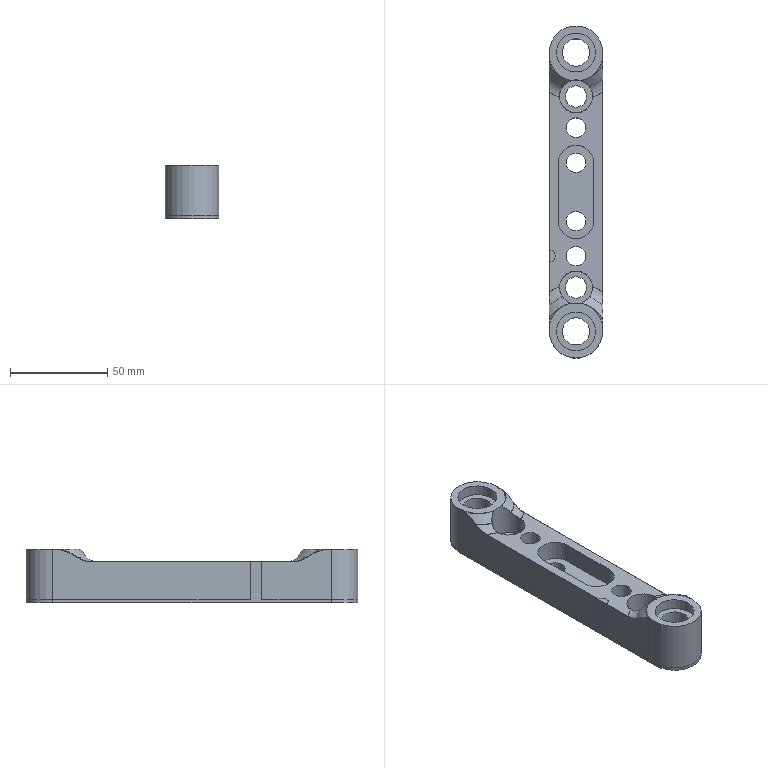NC program | NX | posted with a generic post | part box 27.4 x 170.48 x 27.5 mm
Lines 1 to 377 of 16455:
N10 G17 G21 G94 G90
(PLANAR_MILL_COPY , TOOL : D50R0.8)
N12 T01 M6
N14 G54
N16 G17 G0 G90 X120. Y0. B0. C0. S2000 M3
N18 G43 Z30. H1
N20 Z2.05
N22 G94 G1 Z0.05 F800.
N24 X90.
N26 X-90.
N28 X-120.
N30 Z2.05
N32 G0 Z30.
(PLANAR_MILL_COPY_COPY , TOOL : D50R0.8)
N34 X120.
N36 Z2.
N38 G1 Z0.
N40 X90.
N42 X-90.
N44 X-120.
N46 Z2.
N48 G0 Z30.
N50 M5
(FLOOR_FACING_COPY , TOOL : D12开粗)
N52 T05 M6
N54 G54
N56 G17 G0 G90 X0. Y22.7 B0. C0. S3000 M3
N58 G43 Z30. H5
N60 Z-3.4
N62 G94 G1 Z-6.4 F800.
N64 Y10.7
N66 X44.314
N68 X44.221 Y10.46
N70 G3 X44.221 Y-10.46 R11.5
N72 G1 X44.314 Y-10.7
N74 X-44.314
N76 X-44.221 Y-10.46
N78 G3 X-44.221 Y10.46 R11.5
N80 G1 X-44.314 Y10.7
N82 X0.
N84 Y1.7
N86 X28.571
N88 G3 X28.571 Y-1.7 R20.5
N90 G1 X-28.571
N92 G3 X-28.571 Y1.7 R20.5
N94 G1 X0.
N96 X1.
N98 Y22.7
N100 Z-3.4
N102 G0 Z30.
(PLANAR_MILL_8_COPY , TOOL : D12开粗)
N104 X-45.696 Y19.829
N106 Z-4.4
N108 G1 Z-6.4
N110 G3 X-46.236 Y17.053 R2.
N112 G2 X-46.236 Y-17.053 R30.514
N114 G3 X-45.696 Y-19.829 R2.
N116 G1 Z-4.4
N118 G0 Z30.
N120 X45.696
N122 Z-4.4
N124 G1 Z-6.4
N126 G3 X46.236 Y-17.053 R2.
N128 G2 X46.236 Y17.053 R30.514
N130 G3 X45.696 Y19.829 R2.
N132 G1 Z-4.4
N134 G0 Z30.
N136 M5
(PLANAR_MILL_1_COPY , TOOL : D12精光)
N138 T07 M6
N140 G54
N142 G17 G0 G90 X73.505 Y-21.897 B0. C0. S3000 M3
N144 G43 Z30. H7
N146 Z-25.5
N148 G94 G1 Z-27.5 F800.
N150 G41 X73.54 Y-21.7 D7
N152 G3 X71.54 Y-19.7 R2.
N154 G1 X-71.54
N156 G2 X-91.24 Y0. R19.7
N158 X-71.54 Y19.7 R19.7
N160 G1 X71.54
N162 G2 X91.24 Y0. R19.7
N164 X71.54 Y-19.7 R19.7
N166 G3 X69.54 Y-21.7 R2.
N168 G40
N170 G1 X69.575 Y-21.897
N172 X73.505
N174 G41 X73.54 Y-21.7
N176 G3 X71.54 Y-19.7 R2.
N178 G1 X-71.54
N180 G2 X-91.24 Y0. R19.7
N182 X-71.54 Y19.7 R19.7
N184 G1 X71.54
N186 G2 X91.24 Y0. R19.7
N188 X71.54 Y-19.7 R19.7
N190 G3 X69.54 Y-21.7 R2.
N192 G40
N194 G1 X69.575 Y-21.897
N196 Z-25.5
N198 G0 Z30.
(FLOOR_FACING , TOOL : D12精光)
N200 X0. Y22.7
N202 Z-3.5
N204 G1 Z-6.5
N206 Y10.7
N208 X42.964
N210 X42.914 Y10.565
N212 X42.521 Y9.501
N214 G3 X42.521 Y-9.501 R11.5
N216 G1 X42.914 Y-10.565
N218 X42.964 Y-10.7
N220 X-42.964
N222 X-42.914 Y-10.565
N224 X-42.521 Y-9.501
N226 G3 X-42.521 Y9.501 R11.5
N228 G1 X-42.914 Y10.565
N230 X-42.964 Y10.7
N232 X0.
N234 Y1.7
N236 X28.571
N238 G3 X28.571 Y-1.7 R20.5
N240 G1 X-28.571
N242 G3 X-28.571 Y1.7 R20.5
N244 G1 X0.
N246 X1.
N248 Y22.7
N250 Z-3.5
N252 G0 Z30.
(PLANAR_MILL_8 , TOOL : D12精光)
N254 X-45.696 Y19.829
N256 Z-4.5
N258 G1 Z-6.5
N260 G3 X-46.236 Y17.053 R2.
N262 G2 X-46.236 Y-17.053 R30.514
N264 G3 X-45.696 Y-19.829 R2.
N266 G1 Z-4.5
N268 G0 Z30.
N270 X45.696
N272 Z-4.5
N274 G1 Z-6.5
N276 G3 X46.236 Y-17.053 R2.
N278 G2 X46.236 Y17.053 R30.514
N280 G3 X45.696 Y19.829 R2.
N282 G1 Z-4.5
N284 G0 Z30.
N286 M5
(PLANAR_MILL_9_COPY_1 , TOOL : D8精光)
N288 T08 M6
N290 G54
N292 G17 G0 G90 X-14. Y0.6 B0. C0. S3000 M3
N294 G43 Z30. H8
N296 Z-14.4
N298 G94 G1 Z-16.4 F800.
N300 G3 X-15. Y1.6 R1.
N302 X-16.6 Y0. R1.6
N304 X-15. Y-1.6 R1.6
N306 G1 X15.
N308 G3 X16.6 Y0. R1.6
N310 X15. Y1.6 R1.6
N312 G1 X-15.
N314 Y4.8
N316 G3 X-19.8 Y0. R4.8
N318 X-15. Y-4.8 R4.8
N320 G1 X15.
N322 G3 X19.8 Y0. R4.8
N324 X15. Y4.8 R4.8
N326 G1 X-15.
N328 G3 X-16. Y3.8 R1.
N330 G1 Z-14.4
N332 G0 Z30.
(PLANAR_MILL_9 , TOOL : D8精光)
N334 X-14. Y0.7
N336 Z-14.5
N338 G1 Z-16.5
N340 G3 X-15. Y1.7 R1.
N342 X-16.7 Y0. R1.7
N344 X-15. Y-1.7 R1.7
N346 G1 X15.
N348 G3 X16.7 Y0. R1.7
N350 X15. Y1.7 R1.7
N352 G1 X-15.
N354 Y4.9
N356 G3 X-19.9 Y0. R4.9
N358 X-15. Y-4.9 R4.9
N360 G1 X15.
N362 G3 X19.9 Y0. R4.9
N364 X15. Y4.9 R4.9
N366 G1 X-15.
N368 G3 X-16. Y3.9 R1.
N370 G1 Z-14.5
N372 G0 Z30.
(PLANAR_MILL_9_COPY , TOOL : D8精光)
N374 X-15. Y0.
N376 Z-14.5
N378 G1 Z-16.5
N380 G41 X-18. Y2. D8
N382 G3 X-20. Y0. R2.
N384 X-15. Y-5. R5.
N386 G1 X15.
N388 G3 X20. Y0. R5.
N390 X15. Y5. R5.
N392 G1 X-15.
N394 G3 X-20. Y0. R5.
N396 X-18. Y-2. R2.
N398 G40
N400 G1 X-17.803 Y-1.965
N402 Y1.965
N404 G41 X-18. Y2.
N406 G3 X-20. Y0. R2.
N408 X-15. Y-5. R5.
N410 G1 X15.
N412 G3 X20. Y0. R5.
N414 X15. Y5. R5.
N416 G1 X-15.
N418 G3 X-20. Y0. R5.
N420 X-18. Y-2. R2.
N422 G40
N424 G1 X-15. Y0.
N426 Z-14.5
N428 G0 Z30.
N430 M5
(PLANAR_MILL_13_COPY_1 , TOOL : D8开粗)
N432 T19 M6
N434 G54
N436 G17 G0 G90 X-69.557 Y2.056 B0. C0. S3000 M3
N438 G43 Z30. H19
N440 Z-3.5
N442 G94 G1 Z-5.5 F600.
N444 G41 X-69.54 Y2.155 D19
N446 Y3.94
N448 G3 X-71.54 Y5.94 R2.
N450 X-77.48 Y0. R5.94
N452 X-71.54 Y5.94 R-5.94
N454 X-73.54 Y3.94 R2.
N456 G40
N458 G1 X-73.523 Y3.842
N460 X-69.557
N462 G41 X-69.54 Y3.94
N464 G3 X-71.54 Y5.94 R2.
N466 X-77.48 Y0. R5.94
N468 X-71.54 Y5.94 R-5.94
N470 X-73.54 Y3.94 R2.
N472 G1 Y2.155
N474 G40
N476 X-73.523 Y2.056
N478 Z-3.5
N480 G0 Z30.
N482 X69.557 Y-2.056
N484 Z-3.5
N486 G1 Z-5.5
N488 G41 X69.54 Y-2.155
N490 Y-3.94
N492 G3 X71.54 Y-5.94 R2.
N494 X77.48 Y0. R5.94
N496 X71.54 Y-5.94 R-5.94
N498 X73.54 Y-3.94 R2.
N500 G40
N502 G1 X73.523 Y-3.842
N504 X69.557
N506 G41 X69.54 Y-3.94
N508 G3 X71.54 Y-5.94 R2.
N510 X77.48 Y0. R5.94
N512 X71.54 Y-5.94 R-5.94
N514 X73.54 Y-3.94 R2.
N516 G1 Y-2.155
N518 G40
N520 X73.523 Y-2.056
N522 Z-3.5
N524 G0 Z30.
(PLANAR_MILL_13 , TOOL : D8开粗)
N526 X-32.67 Y0.291
N528 Z-15.75
N530 G1 Z-17.75
N532 G41 X-32.5 Y0.44
N534 G3 X-33. Y0.94 R0.5
N536 X-33.94 Y0. R0.94
N538 X-33. Y0.94 R-0.94
N540 X-33.5 Y0.44 R0.5
N542 G40
N544 G1 X-33.483 Y0.342
N546 X-32.517
N548 G41 X-32.5 Y0.44
N550 G3 X-33. Y0.94 R0.5
N552 X-33.94 Y0. R0.94
N554 X-33. Y0.94 R-0.94
N556 X-33.5 Y0.44 R0.5
N558 G40
N560 G1 X-33.33 Y0.291
N562 Z-15.75
N564 G0 Z30.
N566 X33.33
N568 Z-15.75
N570 G1 Z-17.75
N572 G41 X33.5 Y0.44
N574 G3 X33. Y0.94 R0.5
N576 X32.06 Y0. R0.94
N578 X33. Y0.94 R-0.94
N580 X32.5 Y0.44 R0.5
N582 G40
N584 G1 X32.517 Y0.342
N586 X33.483
N588 G41 X33.5 Y0.44
N590 G3 X33. Y0.94 R0.5
N592 X32.06 Y0. R0.94
N594 X33. Y0.94 R-0.94
N596 X32.5 Y0.44 R0.5
N598 G40
N600 G1 X32.67 Y0.291
N602 Z-15.75
N604 G0 Z30.
N606 X33.33
N608 Z-27.
N610 G1 Z-29.
N612 G41 X33.5 Y0.44
N614 G3 X33. Y0.94 R0.5
N616 X32.06 Y0. R0.94
N618 X33. Y0.94 R-0.94
N620 X32.5 Y0.44 R0.5
N622 G40
N624 G1 X32.517 Y0.342
N626 X33.483
N628 G41 X33.5 Y0.44
N630 G3 X33. Y0.94 R0.5
N632 X32.06 Y0. R0.94
N634 X33. Y0.94 R-0.94
N636 X32.5 Y0.44 R0.5
N638 G40
N640 G1 X32.67 Y0.291
N642 Z-27.
N644 G0 Z30.
N646 X-32.67
N648 Z-27.
N650 G1 Z-29.
N652 G41 X-32.5 Y0.44
N654 G3 X-33. Y0.94 R0.5
N656 X-33.94 Y0. R0.94
N658 X-33. Y0.94 R-0.94
N660 X-33.5 Y0.44 R0.5
N662 G40
N664 G1 X-33.483 Y0.342
N666 X-32.517
N668 G41 X-32.5 Y0.44
N670 G3 X-33. Y0.94 R0.5
N672 X-33.94 Y0. R0.94
N674 X-33. Y0.94 R-0.94
N676 X-33.5 Y0.44 R0.5
N678 G40
N680 G1 X-33.33 Y0.291
N682 Z-27.
N684 G0 Z30.
N686 M5